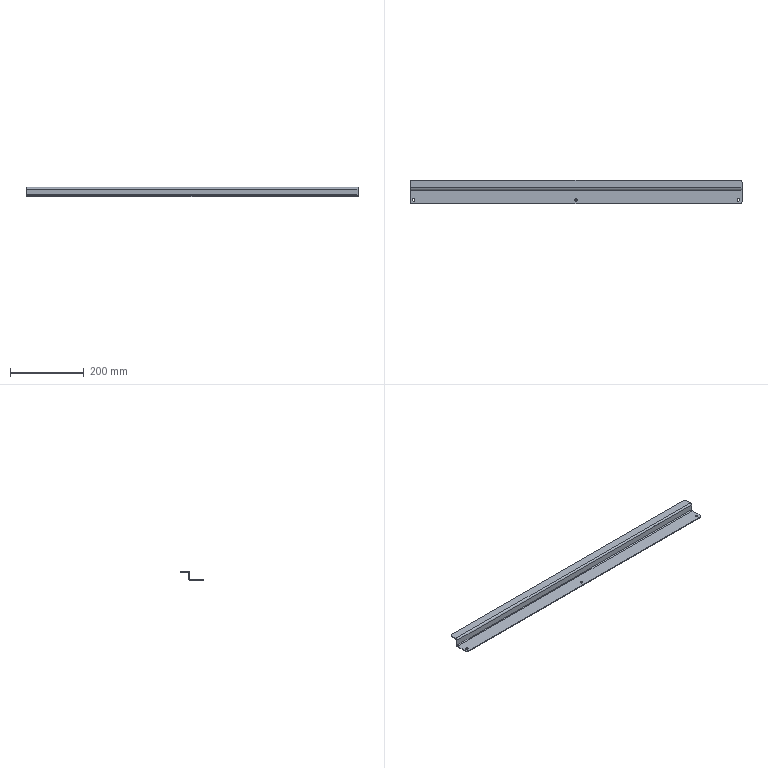Part | STEP file | J451-EBZ05-06-04-Part-1 | 1 solid | 24 faces | box 900 x 62.7 x 25 mm | volume 170348 mm3 | cylinder 14 | plane 10 | commonest cylinder face diameters 6.8 x6 10 x4 4.6 x2 9.2 x2